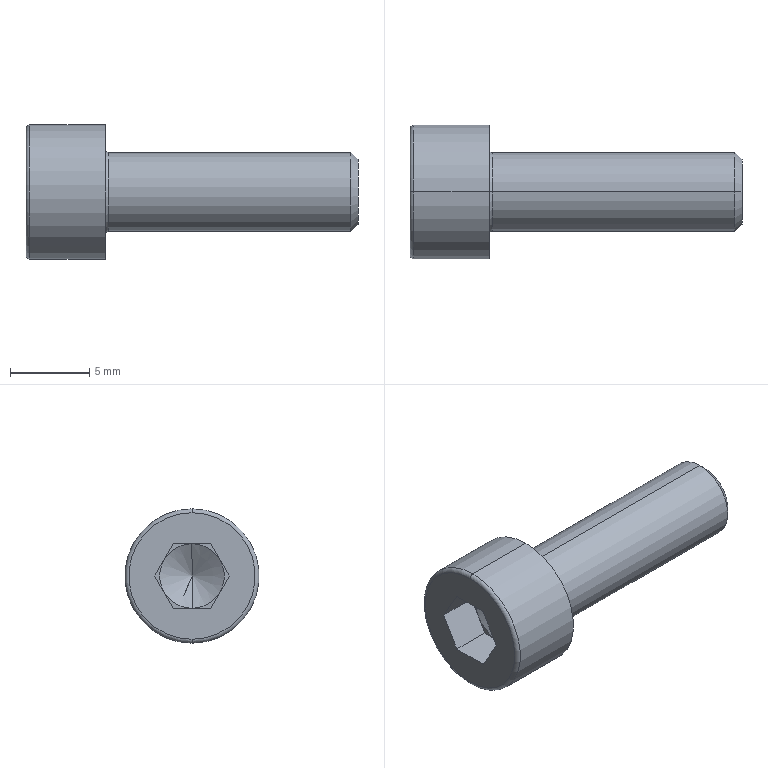Part | SolidWorks | features Fillet 2, RevCut 2, Attribute 1, Cut 1, LPattern 1, Revolution 1 | 1 solid | 27 faces | box 21 x 8.5 x 8.5 mm | volume 554.946 mm3 | plane 15 | cone 4 | torus 4 | cylinder 4 | commonest cylinder face diameters 5 x2 8.5 x2
STEP:
#1=CARTESIAN_POINT('',(3.679,0.,0.));
#2=VERTEX_POINT('',#1);
#3=CARTESIAN_POINT('',(2.5,0.,2.042));
#4=VERTEX_POINT('',#3);
#5=CARTESIAN_POINT('',(2.5,0.,2.042));
#6=DIRECTION('',(-0.5,0.,0.866));
#7=VECTOR('',#6,1000.);
#8=LINE('',#5,#7);
#9=EDGE_CURVE('',#2,#4,#8,.T.);
#10=ORIENTED_EDGE('',*,*,#9,.F.);
#11=CARTESIAN_POINT('',(2.5,0.,-2.042));
#12=VERTEX_POINT('',#11);
#13=CARTESIAN_POINT('',(2.5,0.,-2.042));
#14=DIRECTION('',(-0.5,0.,-0.866));
#15=VECTOR('',#14,1000.);
#16=LINE('',#13,#15);
#17=EDGE_CURVE('',#2,#12,#16,.T.);
#18=ORIENTED_EDGE('',*,*,#17,.T.);
#19=CARTESIAN_POINT('',(2.5,-1.768,-1.021));
#20=VERTEX_POINT('',#19);
#21=CARTESIAN_POINT('',(2.5,0.,0.));
#22=DIRECTION('',(-1.,0.,0.));
#23=DIRECTION('',(0.,0.,1.));
#24=AXIS2_PLACEMENT_3D('',#21,#22,#23);
#25=CIRCLE('',#24,2.042);
#26=EDGE_CURVE('',#12,#20,#25,.T.);
#27=ORIENTED_EDGE('',*,*,#26,.T.);
#28=CARTESIAN_POINT('',(2.5,-1.768,1.021));
#29=VERTEX_POINT('',#28);
#30=CARTESIAN_POINT('',(2.5,0.,0.));
#31=DIRECTION('',(-1.,0.,0.));
#32=DIRECTION('',(0.,0.,1.));
#33=AXIS2_PLACEMENT_3D('',#30,#31,#32);
#34=CIRCLE('',#33,2.042);
#35=EDGE_CURVE('',#20,#29,#34,.T.);
#36=ORIENTED_EDGE('',*,*,#35,.T.);
#37=CARTESIAN_POINT('',(2.5,0.,0.));
#38=DIRECTION('',(-1.,0.,0.));
#39=DIRECTION('',(0.,0.,1.));
#40=AXIS2_PLACEMENT_3D('',#37,#38,#39);
#41=CIRCLE('',#40,2.042);
#42=EDGE_CURVE('',#29,#4,#41,.T.);
#43=ORIENTED_EDGE('',*,*,#42,.T.);
#44=EDGE_LOOP('',(#10,#18,#27,#36,#43));
#45=FACE_OUTER_BOUND('',#44,.T.);
#46=CARTESIAN_POINT('',(2.5,0.,0.));
#47=DIRECTION('',(-1.,0.,0.));
#48=DIRECTION('',(0.,0.,1.));
#49=AXIS2_PLACEMENT_3D('',#46,#47,#48);
#50=CONICAL_SURFACE('',#49,2.042,1.047);
#51=ADVANCED_FACE('',(#45),#50,.F.);
#52=CARTESIAN_POINT('',(0.25,0.,-4.25));
#53=VERTEX_POINT('',#52);
#54=CARTESIAN_POINT('',(0.25,0.,4.25));
#55=VERTEX_POINT('',#54);
#56=CARTESIAN_POINT('',(0.25,0.,0.));
#57=DIRECTION('',(1.,0.,0.));
#58=DIRECTION('',(0.,0.,1.));
#59=AXIS2_PLACEMENT_3D('',#56,#57,#58);
#60=CIRCLE('',#59,4.25);
#61=EDGE_CURVE('',#53,#55,#60,.T.);
#62=ORIENTED_EDGE('',*,*,#61,.F.);
#63=CARTESIAN_POINT('',(0.,0.,-4.));
#64=VERTEX_POINT('',#63);
#65=CARTESIAN_POINT('',(0.25,0.,-4.));
#66=DIRECTION('',(0.,1.,0.));
#67=DIRECTION('',(0.,0.,1.));
#68=AXIS2_PLACEMENT_3D('',#65,#66,#67);
#69=CIRCLE('',#68,0.25);
#70=EDGE_CURVE('',#53,#64,#69,.T.);
#71=ORIENTED_EDGE('',*,*,#70,.T.);
#72=CARTESIAN_POINT('',(0.,0.,4.));
#73=VERTEX_POINT('',#72);
#74=CARTESIAN_POINT('',(0.,0.,0.));
#75=DIRECTION('',(-1.,0.,0.));
#76=DIRECTION('',(0.,0.,1.));
#77=AXIS2_PLACEMENT_3D('',#74,#75,#76);
#78=CIRCLE('',#77,4.);
#79=EDGE_CURVE('',#73,#64,#78,.T.);
#80=ORIENTED_EDGE('',*,*,#79,.F.);
#81=CARTESIAN_POINT('',(0.25,0.,4.));
#82=DIRECTION('',(0.,-1.,0.));
#83=DIRECTION('',(0.,0.,-1.));
#84=AXIS2_PLACEMENT_3D('',#81,#82,#83);
#85=CIRCLE('',#84,0.25);
#86=EDGE_CURVE('',#55,#73,#85,.T.);
#87=ORIENTED_EDGE('',*,*,#86,.F.);
#88=EDGE_LOOP('',(#62,#71,#80,#87));
#89=FACE_OUTER_BOUND('',#88,.T.);
#90=CARTESIAN_POINT('',(0.25,0.,0.));
#91=DIRECTION('',(-1.,0.,0.));
#92=DIRECTION('',(0.,0.,1.));
#93=AXIS2_PLACEMENT_3D('',#90,#91,#92);
#94=TOROIDAL_SURFACE('',#93,4.,0.25);
#95=ADVANCED_FACE('',(#89),#94,.T.);
#96=CARTESIAN_POINT('',(5.2,0.,2.5));
#97=VERTEX_POINT('',#96);
#98=CARTESIAN_POINT('',(5.2,0.,-2.5));
#99=VERTEX_POINT('',#98);
#100=CARTESIAN_POINT('',(5.2,0.,0.));
#101=DIRECTION('',(1.,0.,0.));
#102=DIRECTION('',(0.,0.,-1.));
#103=AXIS2_PLACEMENT_3D('',#100,#101,#102);
#104=CIRCLE('',#103,2.5);
#105=EDGE_CURVE('',#97,#99,#104,.T.);
#106=ORIENTED_EDGE('',*,*,#105,.F.);
#107=CARTESIAN_POINT('',(5.,0.,2.7));
#108=VERTEX_POINT('',#107);
#109=CARTESIAN_POINT('',(5.2,0.,2.7));
#110=DIRECTION('',(0.,1.,0.));
#111=DIRECTION('',(0.,0.,1.));
#112=AXIS2_PLACEMENT_3D('',#109,#110,#111);
#113=CIRCLE('',#112,0.2);
#114=EDGE_CURVE('',#97,#108,#113,.T.);
#115=ORIENTED_EDGE('',*,*,#114,.T.);
#116=CARTESIAN_POINT('',(5.,0.,-2.7));
#117=VERTEX_POINT('',#116);
#118=CARTESIAN_POINT('',(5.,0.,0.));
#119=DIRECTION('',(-1.,0.,0.));
#120=DIRECTION('',(0.,0.,-1.));
#121=AXIS2_PLACEMENT_3D('',#118,#119,#120);
#122=CIRCLE('',#121,2.7);
#123=EDGE_CURVE('',#117,#108,#122,.T.);
#124=ORIENTED_EDGE('',*,*,#123,.F.);
#125=CARTESIAN_POINT('',(5.2,0.,-2.7));
#126=DIRECTION('',(0.,-1.,0.));
#127=DIRECTION('',(0.,0.,-1.));
#128=AXIS2_PLACEMENT_3D('',#125,#126,#127);
#129=CIRCLE('',#128,0.2);
#130=EDGE_CURVE('',#99,#117,#129,.T.);
#131=ORIENTED_EDGE('',*,*,#130,.F.);
#132=EDGE_LOOP('',(#106,#115,#124,#131));
#133=FACE_OUTER_BOUND('',#132,.T.);
#134=CARTESIAN_POINT('',(5.2,0.,0.));
#135=DIRECTION('',(1.,0.,0.));
#136=DIRECTION('',(0.,0.,-1.));
#137=AXIS2_PLACEMENT_3D('',#134,#135,#136);
#138=TOROIDAL_SURFACE('',#137,2.7,0.2);
#139=ADVANCED_FACE('',(#133),#138,.F.);
#140=CARTESIAN_POINT('',(21.,0.,2.055));
#141=VERTEX_POINT('',#140);
#142=CARTESIAN_POINT('',(21.,0.,-2.055));
#143=VERTEX_POINT('',#142);
#144=CARTESIAN_POINT('',(21.,0.,0.));
#145=DIRECTION('',(-1.,0.,0.));
#146=DIRECTION('',(0.,0.,1.));
#147=AXIS2_PLACEMENT_3D('',#144,#145,#146);
#148=CIRCLE('',#147,2.055);
#149=EDGE_CURVE('',#141,#143,#148,.T.);
#150=ORIENTED_EDGE('',*,*,#149,.T.);
#151=CARTESIAN_POINT('',(20.555,0.,-2.5));
#152=VERTEX_POINT('',#151);
#153=CARTESIAN_POINT('',(21.,0.,-2.055));
#154=DIRECTION('',(-0.7071,0.,-0.7071));
#155=VECTOR('',#154,1000.);
#156=LINE('',#153,#155);
#157=EDGE_CURVE('',#143,#152,#156,.T.);
#158=ORIENTED_EDGE('',*,*,#157,.T.);
#159=CARTESIAN_POINT('',(20.555,0.,2.5));
#160=VERTEX_POINT('',#159);
#161=CARTESIAN_POINT('',(20.555,0.,0.));
#162=DIRECTION('',(-1.,0.,0.));
#163=DIRECTION('',(0.,0.,1.));
#164=AXIS2_PLACEMENT_3D('',#161,#162,#163);
#165=CIRCLE('',#164,2.5);
#166=EDGE_CURVE('',#160,#152,#165,.T.);
#167=ORIENTED_EDGE('',*,*,#166,.F.);
#168=CARTESIAN_POINT('',(21.,0.,2.055));
#169=DIRECTION('',(-0.7071,0.,0.7071));
#170=VECTOR('',#169,1000.);
#171=LINE('',#168,#170);
#172=EDGE_CURVE('',#141,#160,#171,.T.);
#173=ORIENTED_EDGE('',*,*,#172,.F.);
#174=EDGE_LOOP('',(#150,#158,#167,#173));
#175=FACE_OUTER_BOUND('',#174,.T.);
#176=CARTESIAN_POINT('',(21.,0.,0.));
#177=DIRECTION('',(-1.,0.,0.));
#178=DIRECTION('',(0.,0.,1.));
#179=AXIS2_PLACEMENT_3D('',#176,#177,#178);
#180=CONICAL_SURFACE('',#179,2.055,0.7854);
#181=ADVANCED_FACE('',(#175),#180,.T.);
#182=ORIENTED_EDGE('',*,*,#166,.T.);
#183=CARTESIAN_POINT('',(-31.75,0.,-2.5));
#184=DIRECTION('',(-1.,0.,0.));
#185=VECTOR('',#184,1000.);
#186=LINE('',#183,#185);
#187=EDGE_CURVE('',#152,#99,#186,.T.);
#188=ORIENTED_EDGE('',*,*,#187,.T.);
#189=CARTESIAN_POINT('',(5.2,0.,0.));
#190=DIRECTION('',(1.,0.,0.));
#191=DIRECTION('',(0.,0.,-1.));
#192=AXIS2_PLACEMENT_3D('',#189,#190,#191);
#193=CIRCLE('',#192,2.5);
#194=EDGE_CURVE('',#99,#97,#193,.T.);
#195=ORIENTED_EDGE('',*,*,#194,.T.);
#196=CARTESIAN_POINT('',(-31.75,0.,2.5));
#197=DIRECTION('',(-1.,0.,0.));
#198=VECTOR('',#197,1000.);
#199=LINE('',#196,#198);
#200=EDGE_CURVE('',#160,#97,#199,.T.);
#201=ORIENTED_EDGE('',*,*,#200,.F.);
#202=EDGE_LOOP('',(#182,#188,#195,#201));
#203=FACE_OUTER_BOUND('',#202,.T.);
#204=CARTESIAN_POINT('',(-31.75,0.,0.));
#205=DIRECTION('',(-1.,0.,0.));
#206=DIRECTION('',(0.,0.,1.));
#207=AXIS2_PLACEMENT_3D('',#204,#205,#206);
#208=CYLINDRICAL_SURFACE('',#207,2.5);
#209=ADVANCED_FACE('',(#203),#208,.T.);
#210=CARTESIAN_POINT('',(5.,0.,4.25));
#211=VERTEX_POINT('',#210);
#212=CARTESIAN_POINT('',(5.,0.,-4.25));
#213=VERTEX_POINT('',#212);
#214=CARTESIAN_POINT('',(5.,0.,0.));
#215=DIRECTION('',(-1.,0.,0.));
#216=DIRECTION('',(0.,0.,1.));
#217=AXIS2_PLACEMENT_3D('',#214,#215,#216);
#218=CIRCLE('',#217,4.25);
#219=EDGE_CURVE('',#211,#213,#218,.T.);
#220=ORIENTED_EDGE('',*,*,#219,.T.);
#221=CARTESIAN_POINT('',(-31.75,0.,-4.25));
#222=DIRECTION('',(-1.,0.,0.));
#223=VECTOR('',#222,1000.);
#224=LINE('',#221,#223);
#225=EDGE_CURVE('',#213,#53,#224,.T.);
#226=ORIENTED_EDGE('',*,*,#225,.T.);
#227=ORIENTED_EDGE('',*,*,#61,.T.);
#228=CARTESIAN_POINT('',(-31.75,0.,4.25));
#229=DIRECTION('',(-1.,0.,0.));
#230=VECTOR('',#229,1000.);
#231=LINE('',#228,#230);
#232=EDGE_CURVE('',#211,#55,#231,.T.);
#233=ORIENTED_EDGE('',*,*,#232,.F.);
#234=EDGE_LOOP('',(#220,#226,#227,#233));
#235=FACE_OUTER_BOUND('',#234,.T.);
#236=CARTESIAN_POINT('',(-31.75,0.,0.));
#237=DIRECTION('',(-1.,0.,0.));
#238=DIRECTION('',(0.,0.,1.));
#239=AXIS2_PLACEMENT_3D('',#236,#237,#238);
#240=CYLINDRICAL_SURFACE('',#239,4.25);
#241=ADVANCED_FACE('',(#235),#240,.T.);
#242=CARTESIAN_POINT('',(0.,2.358,0.));
#243=VERTEX_POINT('',#242);
#244=CARTESIAN_POINT('',(0.,1.179,2.042));
#245=VERTEX_POINT('',#244);
#246=CARTESIAN_POINT('',(0.,2.358,0.));
#247=DIRECTION('',(0.,-0.5,0.866));
#248=VECTOR('',#247,1000.);
#249=LINE('',#246,#248);
#250=EDGE_CURVE('',#243,#245,#249,.T.);
#251=ORIENTED_EDGE('',*,*,#250,.T.);
#252=CARTESIAN_POINT('',(0.,-1.179,2.042));
#253=VERTEX_POINT('',#252);
#254=CARTESIAN_POINT('',(0.,-1.179,2.042));
#255=DIRECTION('',(0.,1.,0.));
#256=VECTOR('',#255,1000.);
#257=LINE('',#254,#256);
#258=EDGE_CURVE('',#253,#245,#257,.T.);
#259=ORIENTED_EDGE('',*,*,#258,.F.);
#260=CARTESIAN_POINT('',(0.,-2.358,0.));
#261=VERTEX_POINT('',#260);
#262=CARTESIAN_POINT('',(0.,-1.179,2.042));
#263=DIRECTION('',(0.,-0.5,-0.866));
#264=VECTOR('',#263,1000.);
#265=LINE('',#262,#264);
#266=EDGE_CURVE('',#253,#261,#265,.T.);
#267=ORIENTED_EDGE('',*,*,#266,.T.);
#268=CARTESIAN_POINT('',(0.,-1.179,-2.042));
#269=VERTEX_POINT('',#268);
#270=CARTESIAN_POINT('',(0.,-2.358,0.));
#271=DIRECTION('',(0.,0.5,-0.866));
#272=VECTOR('',#271,1000.);
#273=LINE('',#270,#272);
#274=EDGE_CURVE('',#261,#269,#273,.T.);
#275=ORIENTED_EDGE('',*,*,#274,.T.);
#276=CARTESIAN_POINT('',(0.,1.179,-2.042));
#277=VERTEX_POINT('',#276);
#278=CARTESIAN_POINT('',(0.,1.179,-2.042));
#279=DIRECTION('',(0.,-1.,0.));
#280=VECTOR('',#279,1000.);
#281=LINE('',#278,#280);
#282=EDGE_CURVE('',#277,#269,#281,.T.);
#283=ORIENTED_EDGE('',*,*,#282,.F.);
#284=CARTESIAN_POINT('',(0.,2.358,0.));
#285=DIRECTION('',(0.,-0.5,-0.866));
#286=VECTOR('',#285,1000.);
#287=LINE('',#284,#286);
#288=EDGE_CURVE('',#243,#277,#287,.T.);
#289=ORIENTED_EDGE('',*,*,#288,.F.);
#290=EDGE_LOOP('',(#251,#259,#267,#275,#283,#289));
#291=FACE_BOUND('',#290,.T.);
#292=ORIENTED_EDGE('',*,*,#79,.T.);
#293=CARTESIAN_POINT('',(0.,0.,0.));
#294=DIRECTION('',(-1.,0.,0.));
#295=DIRECTION('',(0.,0.,1.));
#296=AXIS2_PLACEMENT_3D('',#293,#294,#295);
#297=CIRCLE('',#296,4.);
#298=EDGE_CURVE('',#64,#73,#297,.T.);
#299=ORIENTED_EDGE('',*,*,#298,.T.);
#300=EDGE_LOOP('',(#292,#299));
#301=FACE_OUTER_BOUND('',#300,.T.);
#302=CARTESIAN_POINT('',(0.,0.,0.));
#303=DIRECTION('',(-1.,0.,0.));
#304=DIRECTION('',(0.,0.,1.));
#305=AXIS2_PLACEMENT_3D('',#302,#303,#304);
#306=PLANE('',#305);
#307=ADVANCED_FACE('',(#291,#301),#306,.T.);
#308=ORIENTED_EDGE('',*,*,#225,.F.);
#309=CARTESIAN_POINT('',(5.,0.,0.));
#310=DIRECTION('',(-1.,0.,0.));
#311=DIRECTION('',(0.,0.,1.));
#312=AXIS2_PLACEMENT_3D('',#309,#310,#311);
#313=CIRCLE('',#312,4.25);
#314=EDGE_CURVE('',#213,#211,#313,.T.);
#315=ORIENTED_EDGE('',*,*,#314,.T.);
#316=ORIENTED_EDGE('',*,*,#232,.T.);
#317=CARTESIAN_POINT('',(0.25,0.,0.));
#318=DIRECTION('',(1.,0.,0.));
#319=DIRECTION('',(0.,0.,1.));
#320=AXIS2_PLACEMENT_3D('',#317,#318,#319);
#321=CIRCLE('',#320,4.25);
#322=EDGE_CURVE('',#55,#53,#321,.T.);
#323=ORIENTED_EDGE('',*,*,#322,.T.);
#324=EDGE_LOOP('',(#308,#315,#316,#323));
#325=FACE_OUTER_BOUND('',#324,.T.);
#326=CARTESIAN_POINT('',(-31.75,0.,0.));
#327=DIRECTION('',(-1.,0.,0.));
#328=DIRECTION('',(0.,0.,1.));
#329=AXIS2_PLACEMENT_3D('',#326,#327,#328);
#330=CYLINDRICAL_SURFACE('',#329,4.25);
#331=ADVANCED_FACE('',(#325),#330,.T.);
#332=ORIENTED_EDGE('',*,*,#123,.T.);
#333=CARTESIAN_POINT('',(5.,0.,0.));
#334=DIRECTION('',(-1.,0.,0.));
#335=DIRECTION('',(0.,0.,-1.));
#336=AXIS2_PLACEMENT_3D('',#333,#334,#335);
#337=CIRCLE('',#336,2.7);
#338=EDGE_CURVE('',#108,#117,#337,.T.);
#339=ORIENTED_EDGE('',*,*,#338,.T.);
#340=EDGE_LOOP('',(#332,#339));
#341=FACE_BOUND('',#340,.T.);
#342=ORIENTED_EDGE('',*,*,#219,.F.);
#343=ORIENTED_EDGE('',*,*,#314,.F.);
#344=EDGE_LOOP('',(#342,#343));
#345=FACE_OUTER_BOUND('',#344,.T.);
#346=CARTESIAN_POINT('',(5.,4.25,0.));
#347=DIRECTION('',(1.,0.,0.));
#348=DIRECTION('',(0.,0.,-1.));
#349=AXIS2_PLACEMENT_3D('',#346,#347,#348);
#350=PLANE('',#349);
#351=ADVANCED_FACE('',(#341,#345),#350,.T.);
#352=ORIENTED_EDGE('',*,*,#187,.F.);
#353=CARTESIAN_POINT('',(20.555,0.,0.));
#354=DIRECTION('',(-1.,0.,0.));
#355=DIRECTION('',(0.,0.,1.));
#356=AXIS2_PLACEMENT_3D('',#353,#354,#355);
#357=CIRCLE('',#356,2.5);
#358=EDGE_CURVE('',#152,#160,#357,.T.);
#359=ORIENTED_EDGE('',*,*,#358,.T.);
#360=ORIENTED_EDGE('',*,*,#200,.T.);
#361=ORIENTED_EDGE('',*,*,#105,.T.);
#362=EDGE_LOOP('',(#352,#359,#360,#361));
#363=FACE_OUTER_BOUND('',#362,.T.);
#364=CARTESIAN_POINT('',(-31.75,0.,0.));
#365=DIRECTION('',(-1.,0.,0.));
#366=DIRECTION('',(0.,0.,1.));
#367=AXIS2_PLACEMENT_3D('',#364,#365,#366);
#368=CYLINDRICAL_SURFACE('',#367,2.5);
#369=ADVANCED_FACE('',(#363),#368,.T.);
#370=ORIENTED_EDGE('',*,*,#157,.F.);
#371=CARTESIAN_POINT('',(21.,0.,0.));
#372=DIRECTION('',(-1.,0.,0.));
#373=DIRECTION('',(0.,0.,1.));
#374=AXIS2_PLACEMENT_3D('',#371,#372,#373);
#375=CIRCLE('',#374,2.055);
#376=EDGE_CURVE('',#143,#141,#375,.T.);
#377=ORIENTED_EDGE('',*,*,#376,.T.);
#378=ORIENTED_EDGE('',*,*,#172,.T.);
#379=ORIENTED_EDGE('',*,*,#358,.F.);
#380=EDGE_LOOP('',(#370,#377,#378,#379));
#381=FACE_OUTER_BOUND('',#380,.T.);
#382=CARTESIAN_POINT('',(21.,0.,0.));
#383=DIRECTION('',(-1.,0.,0.));
#384=DIRECTION('',(0.,0.,1.));
#385=AXIS2_PLACEMENT_3D('',#382,#383,#384);
#386=CONICAL_SURFACE('',#385,2.055,0.7854);
#387=ADVANCED_FACE('',(#381),#386,.T.);
#388=ORIENTED_EDGE('',*,*,#149,.F.);
#389=ORIENTED_EDGE('',*,*,#376,.F.);
#390=EDGE_LOOP('',(#388,#389));
#391=FACE_OUTER_BOUND('',#390,.T.);
#392=CARTESIAN_POINT('',(21.,2.055,0.));
#393=DIRECTION('',(1.,0.,0.));
#394=DIRECTION('',(0.,0.,-1.));
#395=AXIS2_PLACEMENT_3D('',#392,#393,#394);
#396=PLANE('',#395);
#397=ADVANCED_FACE('',(#391),#396,.T.);
#398=ORIENTED_EDGE('',*,*,#114,.F.);
#399=ORIENTED_EDGE('',*,*,#194,.F.);
#400=ORIENTED_EDGE('',*,*,#130,.T.);
#401=ORIENTED_EDGE('',*,*,#338,.F.);
#402=EDGE_LOOP('',(#398,#399,#400,#401));
#403=FACE_OUTER_BOUND('',#402,.T.);
#404=CARTESIAN_POINT('',(5.2,0.,0.));
#405=DIRECTION('',(1.,0.,0.));
#406=DIRECTION('',(0.,0.,-1.));
#407=AXIS2_PLACEMENT_3D('',#404,#405,#406);
#408=TOROIDAL_SURFACE('',#407,2.7,0.2);
#409=ADVANCED_FACE('',(#403),#408,.F.);
#410=ORIENTED_EDGE('',*,*,#70,.F.);
#411=ORIENTED_EDGE('',*,*,#322,.F.);
#412=ORIENTED_EDGE('',*,*,#86,.T.);
#413=ORIENTED_EDGE('',*,*,#298,.F.);
#414=EDGE_LOOP('',(#410,#411,#412,#413));
#415=FACE_OUTER_BOUND('',#414,.T.);
#416=CARTESIAN_POINT('',(0.25,0.,0.));
#417=DIRECTION('',(-1.,0.,0.));
#418=DIRECTION('',(0.,0.,1.));
#419=AXIS2_PLACEMENT_3D('',#416,#417,#418);
#420=TOROIDAL_SURFACE('',#419,4.,0.25);
#421=ADVANCED_FACE('',(#415),#420,.T.);
#422=ORIENTED_EDGE('',*,*,#250,.F.);
#423=CARTESIAN_POINT('',(2.5,2.358,0.));
#424=VERTEX_POINT('',#423);
#425=CARTESIAN_POINT('',(2.5,2.358,0.));
#426=DIRECTION('',(-1.,0.,0.));
#427=VECTOR('',#426,1000.);
#428=LINE('',#425,#427);
#429=EDGE_CURVE('',#424,#243,#428,.T.);
#430=ORIENTED_EDGE('',*,*,#429,.F.);
#431=CARTESIAN_POINT('',(2.5,1.768,1.021));
#432=VERTEX_POINT('',#431);
#433=CARTESIAN_POINT('',(2.5,2.358,0.));
#434=DIRECTION('',(0.,-0.5,0.866));
#435=VECTOR('',#434,1000.);
#436=LINE('',#433,#435);
#437=EDGE_CURVE('',#424,#432,#436,.T.);
#438=ORIENTED_EDGE('',*,*,#437,.T.);
#439=CARTESIAN_POINT('',(2.5,1.179,2.042));
#440=VERTEX_POINT('',#439);
#441=CARTESIAN_POINT('',(2.5,2.358,0.));
#442=DIRECTION('',(0.,-0.5,0.866));
#443=VECTOR('',#442,1000.);
#444=LINE('',#441,#443);
#445=EDGE_CURVE('',#432,#440,#444,.T.);
#446=ORIENTED_EDGE('',*,*,#445,.T.);
#447=CARTESIAN_POINT('',(2.5,1.179,2.042));
#448=DIRECTION('',(-1.,0.,0.));
#449=VECTOR('',#448,1000.);
#450=LINE('',#447,#449);
#451=EDGE_CURVE('',#440,#245,#450,.T.);
#452=ORIENTED_EDGE('',*,*,#451,.T.);
#453=EDGE_LOOP('',(#422,#430,#438,#446,#452));
#454=FACE_OUTER_BOUND('',#453,.T.);
#455=CARTESIAN_POINT('',(2.5,2.358,0.));
#456=DIRECTION('',(0.,-0.866,-0.5));
#457=DIRECTION('',(0.,0.5,-0.866));
#458=AXIS2_PLACEMENT_3D('',#455,#456,#457);
#459=PLANE('',#458);
#460=ADVANCED_FACE('',(#454),#459,.T.);
#461=ORIENTED_EDGE('',*,*,#258,.T.);
#462=ORIENTED_EDGE('',*,*,#451,.F.);
#463=CARTESIAN_POINT('',(2.5,-1.179,2.042));
#464=DIRECTION('',(0.,1.,0.));
#465=VECTOR('',#464,1000.);
#466=LINE('',#463,#465);
#467=EDGE_CURVE('',#4,#440,#466,.T.);
#468=ORIENTED_EDGE('',*,*,#467,.F.);
#469=CARTESIAN_POINT('',(2.5,-1.179,2.042));
#470=VERTEX_POINT('',#469);
#471=CARTESIAN_POINT('',(2.5,-1.179,2.042));
#472=DIRECTION('',(0.,1.,0.));
#473=VECTOR('',#472,1000.);
#474=LINE('',#471,#473);
#475=EDGE_CURVE('',#470,#4,#474,.T.);
#476=ORIENTED_EDGE('',*,*,#475,.F.);
#477=CARTESIAN_POINT('',(2.5,-1.179,2.042));
#478=DIRECTION('',(-1.,0.,0.));
#479=VECTOR('',#478,1000.);
#480=LINE('',#477,#479);
#481=EDGE_CURVE('',#470,#253,#480,.T.);
#482=ORIENTED_EDGE('',*,*,#481,.T.);
#483=EDGE_LOOP('',(#461,#462,#468,#476,#482));
#484=FACE_OUTER_BOUND('',#483,.T.);
#485=CARTESIAN_POINT('',(2.5,-1.179,2.042));
#486=DIRECTION('',(0.,0.,1.));
#487=DIRECTION('',(0.,-1.,0.));
#488=AXIS2_PLACEMENT_3D('',#485,#486,#487);
#489=PLANE('',#488);
#490=ADVANCED_FACE('',(#484),#489,.F.);
#491=ORIENTED_EDGE('',*,*,#266,.F.);
#492=ORIENTED_EDGE('',*,*,#481,.F.);
#493=CARTESIAN_POINT('',(2.5,-1.179,2.042));
#494=DIRECTION('',(0.,-0.5,-0.866));
#495=VECTOR('',#494,1000.);
#496=LINE('',#493,#495);
#497=EDGE_CURVE('',#470,#29,#496,.T.);
#498=ORIENTED_EDGE('',*,*,#497,.T.);
#499=CARTESIAN_POINT('',(2.5,-2.358,0.));
#500=VERTEX_POINT('',#499);
#501=CARTESIAN_POINT('',(2.5,-1.179,2.042));
#502=DIRECTION('',(0.,-0.5,-0.866));
#503=VECTOR('',#502,1000.);
#504=LINE('',#501,#503);
#505=EDGE_CURVE('',#29,#500,#504,.T.);
#506=ORIENTED_EDGE('',*,*,#505,.T.);
#507=CARTESIAN_POINT('',(2.5,-2.358,0.));
#508=DIRECTION('',(-1.,0.,0.));
#509=VECTOR('',#508,1000.);
#510=LINE('',#507,#509);
#511=EDGE_CURVE('',#500,#261,#510,.T.);
#512=ORIENTED_EDGE('',*,*,#511,.T.);
#513=EDGE_LOOP('',(#491,#492,#498,#506,#512));
#514=FACE_OUTER_BOUND('',#513,.T.);
#515=CARTESIAN_POINT('',(2.5,-1.179,2.042));
#516=DIRECTION('',(0.,0.866,-0.5));
#517=DIRECTION('',(0.,0.5,0.866));
#518=AXIS2_PLACEMENT_3D('',#515,#516,#517);
#519=PLANE('',#518);
#520=ADVANCED_FACE('',(#514),#519,.T.);
#521=ORIENTED_EDGE('',*,*,#274,.F.);
#522=ORIENTED_EDGE('',*,*,#511,.F.);
#523=CARTESIAN_POINT('',(2.5,-2.358,0.));
#524=DIRECTION('',(0.,0.5,-0.866));
#525=VECTOR('',#524,1000.);
#526=LINE('',#523,#525);
#527=EDGE_CURVE('',#500,#20,#526,.T.);
#528=ORIENTED_EDGE('',*,*,#527,.T.);
#529=CARTESIAN_POINT('',(2.5,-1.179,-2.042));
#530=VERTEX_POINT('',#529);
#531=CARTESIAN_POINT('',(2.5,-2.358,0.));
#532=DIRECTION('',(0.,0.5,-0.866));
#533=VECTOR('',#532,1000.);
#534=LINE('',#531,#533);
#535=EDGE_CURVE('',#20,#530,#534,.T.);
#536=ORIENTED_EDGE('',*,*,#535,.T.);
#537=CARTESIAN_POINT('',(2.5,-1.179,-2.042));
#538=DIRECTION('',(-1.,0.,0.));
#539=VECTOR('',#538,1000.);
#540=LINE('',#537,#539);
#541=EDGE_CURVE('',#530,#269,#540,.T.);
#542=ORIENTED_EDGE('',*,*,#541,.T.);
#543=EDGE_LOOP('',(#521,#522,#528,#536,#542));
#544=FACE_OUTER_BOUND('',#543,.T.);
#545=CARTESIAN_POINT('',(2.5,-2.358,0.));
#546=DIRECTION('',(0.,0.866,0.5));
#547=DIRECTION('',(0.,-0.5,0.866));
#548=AXIS2_PLACEMENT_3D('',#545,#546,#547);
#549=PLANE('',#548);
#550=ADVANCED_FACE('',(#544),#549,.T.);
#551=ORIENTED_EDGE('',*,*,#282,.T.);
#552=ORIENTED_EDGE('',*,*,#541,.F.);
#553=CARTESIAN_POINT('',(2.5,1.179,-2.042));
#554=DIRECTION('',(0.,-1.,0.));
#555=VECTOR('',#554,1000.);
#556=LINE('',#553,#555);
#557=EDGE_CURVE('',#12,#530,#556,.T.);
#558=ORIENTED_EDGE('',*,*,#557,.F.);
#559=CARTESIAN_POINT('',(2.5,1.179,-2.042));
#560=VERTEX_POINT('',#559);
#561=CARTESIAN_POINT('',(2.5,1.179,-2.042));
#562=DIRECTION('',(0.,-1.,0.));
#563=VECTOR('',#562,1000.);
#564=LINE('',#561,#563);
#565=EDGE_CURVE('',#560,#12,#564,.T.);
#566=ORIENTED_EDGE('',*,*,#565,.F.);
#567=CARTESIAN_POINT('',(2.5,1.179,-2.042));
#568=DIRECTION('',(-1.,0.,0.));
#569=VECTOR('',#568,1000.);
#570=LINE('',#567,#569);
#571=EDGE_CURVE('',#560,#277,#570,.T.);
#572=ORIENTED_EDGE('',*,*,#571,.T.);
#573=EDGE_LOOP('',(#551,#552,#558,#566,#572));
#574=FACE_OUTER_BOUND('',#573,.T.);
#575=CARTESIAN_POINT('',(2.5,1.179,-2.042));
#576=DIRECTION('',(0.,0.,-1.));
#577=DIRECTION('',(0.,1.,0.));
#578=AXIS2_PLACEMENT_3D('',#575,#576,#577);
#579=PLANE('',#578);
#580=ADVANCED_FACE('',(#574),#579,.F.);
#581=ORIENTED_EDGE('',*,*,#288,.T.);
#582=ORIENTED_EDGE('',*,*,#571,.F.);
#583=CARTESIAN_POINT('',(2.5,1.768,-1.021));
#584=VERTEX_POINT('',#583);
#585=CARTESIAN_POINT('',(2.5,2.358,0.));
#586=DIRECTION('',(0.,-0.5,-0.866));
#587=VECTOR('',#586,1000.);
#588=LINE('',#585,#587);
#589=EDGE_CURVE('',#584,#560,#588,.T.);
#590=ORIENTED_EDGE('',*,*,#589,.F.);
#591=CARTESIAN_POINT('',(2.5,2.358,0.));
#592=DIRECTION('',(0.,-0.5,-0.866));
#593=VECTOR('',#592,1000.);
#594=LINE('',#591,#593);
#595=EDGE_CURVE('',#424,#584,#594,.T.);
#596=ORIENTED_EDGE('',*,*,#595,.F.);
#597=ORIENTED_EDGE('',*,*,#429,.T.);
#598=EDGE_LOOP('',(#581,#582,#590,#596,#597));
#599=FACE_OUTER_BOUND('',#598,.T.);
#600=CARTESIAN_POINT('',(2.5,2.358,0.));
#601=DIRECTION('',(0.,0.866,-0.5));
#602=DIRECTION('',(0.,0.5,0.866));
#603=AXIS2_PLACEMENT_3D('',#600,#601,#602);
#604=PLANE('',#603);
#605=ADVANCED_FACE('',(#599),#604,.F.);
#606=ORIENTED_EDGE('',*,*,#42,.F.);
#607=ORIENTED_EDGE('',*,*,#497,.F.);
#608=ORIENTED_EDGE('',*,*,#475,.T.);
#609=EDGE_LOOP('',(#606,#607,#608));
#610=FACE_OUTER_BOUND('',#609,.T.);
#611=CARTESIAN_POINT('',(2.5,1.179,2.042));
#612=DIRECTION('',(-1.,0.,0.));
#613=DIRECTION('',(0.,0.,1.));
#614=AXIS2_PLACEMENT_3D('',#611,#612,#613);
#615=PLANE('',#614);
#616=ADVANCED_FACE('',(#610),#615,.T.);
#617=ORIENTED_EDGE('',*,*,#35,.F.);
#618=ORIENTED_EDGE('',*,*,#527,.F.);
#619=ORIENTED_EDGE('',*,*,#505,.F.);
#620=EDGE_LOOP('',(#617,#618,#619));
#621=FACE_OUTER_BOUND('',#620,.T.);
#622=CARTESIAN_POINT('',(2.5,1.179,2.042));
#623=DIRECTION('',(-1.,0.,0.));
#624=DIRECTION('',(0.,0.,1.));
#625=AXIS2_PLACEMENT_3D('',#622,#623,#624);
#626=PLANE('',#625);
#627=ADVANCED_FACE('',(#621),#626,.T.);
#628=ORIENTED_EDGE('',*,*,#26,.F.);
#629=ORIENTED_EDGE('',*,*,#557,.T.);
#630=ORIENTED_EDGE('',*,*,#535,.F.);
#631=EDGE_LOOP('',(#628,#629,#630));
#632=FACE_OUTER_BOUND('',#631,.T.);
#633=CARTESIAN_POINT('',(2.5,1.179,2.042));
#634=DIRECTION('',(-1.,0.,0.));
#635=DIRECTION('',(0.,0.,1.));
#636=AXIS2_PLACEMENT_3D('',#633,#634,#635);
#637=PLANE('',#636);
#638=ADVANCED_FACE('',(#632),#637,.T.);
#639=CARTESIAN_POINT('',(2.5,0.,0.));
#640=DIRECTION('',(-1.,0.,0.));
#641=DIRECTION('',(0.,0.,1.));
#642=AXIS2_PLACEMENT_3D('',#639,#640,#641);
#643=CIRCLE('',#642,2.042);
#644=EDGE_CURVE('',#584,#12,#643,.T.);
#645=ORIENTED_EDGE('',*,*,#644,.F.);
#646=ORIENTED_EDGE('',*,*,#589,.T.);
#647=ORIENTED_EDGE('',*,*,#565,.T.);
#648=EDGE_LOOP('',(#645,#646,#647));
#649=FACE_OUTER_BOUND('',#648,.T.);
#650=CARTESIAN_POINT('',(2.5,1.179,2.042));
#651=DIRECTION('',(-1.,0.,0.));
#652=DIRECTION('',(0.,0.,1.));
#653=AXIS2_PLACEMENT_3D('',#650,#651,#652);
#654=PLANE('',#653);
#655=ADVANCED_FACE('',(#649),#654,.T.);
#656=CARTESIAN_POINT('',(2.5,0.,0.));
#657=DIRECTION('',(-1.,0.,0.));
#658=DIRECTION('',(0.,0.,1.));
#659=AXIS2_PLACEMENT_3D('',#656,#657,#658);
#660=CIRCLE('',#659,2.042);
#661=EDGE_CURVE('',#432,#584,#660,.T.);
#662=ORIENTED_EDGE('',*,*,#661,.F.);
#663=ORIENTED_EDGE('',*,*,#437,.F.);
#664=ORIENTED_EDGE('',*,*,#595,.T.);
#665=EDGE_LOOP('',(#662,#663,#664));
#666=FACE_OUTER_BOUND('',#665,.T.);
#667=CARTESIAN_POINT('',(2.5,1.179,2.042));
#668=DIRECTION('',(-1.,0.,0.));
#669=DIRECTION('',(0.,0.,1.));
#670=AXIS2_PLACEMENT_3D('',#667,#668,#669);
#671=PLANE('',#670);
#672=ADVANCED_FACE('',(#666),#671,.T.);
#673=CARTESIAN_POINT('',(2.5,0.,0.));
#674=DIRECTION('',(-1.,0.,0.));
#675=DIRECTION('',(0.,0.,1.));
#676=AXIS2_PLACEMENT_3D('',#673,#674,#675);
#677=CIRCLE('',#676,2.042);
#678=EDGE_CURVE('',#4,#432,#677,.T.);
#679=ORIENTED_EDGE('',*,*,#678,.F.);
#680=ORIENTED_EDGE('',*,*,#467,.T.);
#681=ORIENTED_EDGE('',*,*,#445,.F.);
#682=EDGE_LOOP('',(#679,#680,#681));
#683=FACE_OUTER_BOUND('',#682,.T.);
#684=CARTESIAN_POINT('',(2.5,1.179,2.042));
#685=DIRECTION('',(-1.,0.,0.));
#686=DIRECTION('',(0.,0.,1.));
#687=AXIS2_PLACEMENT_3D('',#684,#685,#686);
#688=PLANE('',#687);
#689=ADVANCED_FACE('',(#683),#688,.T.);
#690=ORIENTED_EDGE('',*,*,#17,.F.);
#691=ORIENTED_EDGE('',*,*,#9,.T.);
#692=ORIENTED_EDGE('',*,*,#678,.T.);
#693=ORIENTED_EDGE('',*,*,#661,.T.);
#694=ORIENTED_EDGE('',*,*,#644,.T.);
#695=EDGE_LOOP('',(#690,#691,#692,#693,#694));
#696=FACE_OUTER_BOUND('',#695,.T.);
#697=CARTESIAN_POINT('',(2.5,0.,0.));
#698=DIRECTION('',(-1.,0.,0.));
#699=DIRECTION('',(0.,0.,1.));
#700=AXIS2_PLACEMENT_3D('',#697,#698,#699);
#701=CONICAL_SURFACE('',#700,2.042,1.047);
#702=ADVANCED_FACE('',(#696),#701,.F.);
#703=CLOSED_SHELL('',(#51,#95,#139,#181,#209,#241,#307,#331,#351,#369,#387,#397,#409,#421,#460,#490,#520,#550,#580,#605,#616,#627,#638,#655,#672,#689,#702));
#704=MANIFOLD_SOLID_BREP('',#703);
#705=CARTESIAN_POINT('',(0.,0.,0.));
#706=DIRECTION('',(0.,0.,1.));
#707=DIRECTION('',(1.,0.,0.));
#708=AXIS2_PLACEMENT_3D('',#705,#706,#707);
#709=(LENGTH_UNIT()NAMED_UNIT(*)SI_UNIT(.MILLI.,.METRE.));
#710=UNCERTAINTY_MEASURE_WITH_UNIT(LENGTH_MEASURE(0.00001),#709,'','');
#711=(NAMED_UNIT(*)PLANE_ANGLE_UNIT()SI_UNIT($,.RADIAN.));
#712=(NAMED_UNIT(*)SI_UNIT($,.STERADIAN.)SOLID_ANGLE_UNIT());
#713=(GEOMETRIC_REPRESENTATION_CONTEXT(3)GLOBAL_UNCERTAINTY_ASSIGNED_CONTEXT((#710))GLOBAL_UNIT_ASSIGNED_CONTEXT((#709,#711,#712))REPRESENTATION_CONTEXT('',''));
#714=ADVANCED_BREP_SHAPE_REPRESENTATION('',(#704,#708),#713);